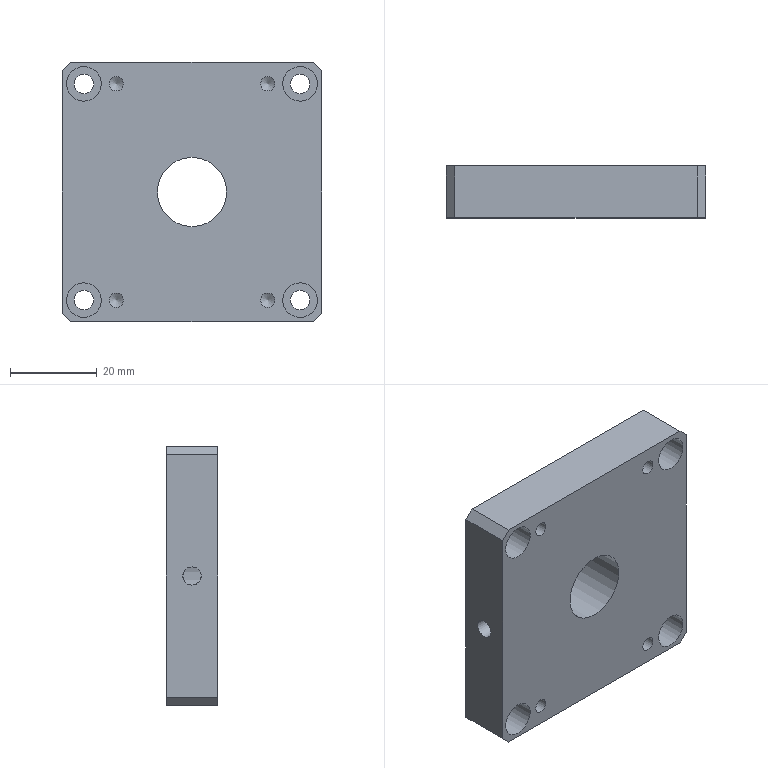CAM job | NX | 3+2 milling, drilling | part box 60 x 12 x 60 mm | stock box 60 x 12 x 60 mm
Tools:
number,name,description,diameter,corner_radius,flute_length,length,flutes
4,D4,平底铣刀-粗,4.0,0.0,25.0,75.0,2
9,D10,平底铣刀-粗,10.0,0.0,35.0,75.0,2
18,D1.5-J,平底铣刀-粗,1.5,0.0,50.0,75.0,2
11,D4-J,平底铣刀-精,4.0,0.0,50.0,75.0,2
10,D10-J,平底铣刀-精,10.0,0.0,35.0,75.0,2
2,D6倒角刀,倒角刀,6.0,0.0,3.0,25.0,2
21,M4X0.7,丝锥,3.3,0.0,35.0,50.0,2
1,C6定点钻,倒角刀,6.0,0.0,3.0,3.0,2
17,ZT1.8,钻头,1.6,0.0,35.0,50.0,2
13,ZT3.4,钻头,3.4,0.0,35.0,50.0,2
11,ZT4.5,钻头,4.5,0.0,35.0,50.0,2
Operations:
program,operation,operation_type,tool,method,geometry_group,spindle_rpm,surface_speed,feed_per_tooth,feed_cut,feed_plunge,cut_length_mm,path_length_mm,cut_time_min,machine_time_min
B,打点-深1_COPY,Operation,C6定点钻,NONE,W-B,3000.0,56.0,0.01,60.0,90.0,3.6,157.71,0.06,0.0754
B,盲锥孔-1-2,Operation,ZT1.8,NONE,W-B,2000.0,12.566,0.0075,30.0,90.0,13.202,176.913,0.4401,0.4564
B,底壁铣螺旋开粗-小_COPY,VolumeBased25DMillingOperation,D1.5-J,分层开粗-切深K-步距G,W-B,6000.0,28.274,0.0167,200.0,100.0,1219.408,1476.121,6.097,6.123
B,NG_钻倒角_2,Operation,D6倒角刀,METHOD,W-B,2000.0,0.0,0.025,100.0,0.0,22.2,303.67,0.222,0.2501
B,平面去毛刺6X45L_COPY_1,SurfaceContour,D6倒角刀,爬面_倒角-切深0-步距G,W-B,3500.0,65.972,0.1429,1000.0,100.0,345.537,759.417,0.3455,0.3869
B,NG_钻倒角_3,Operation,D6倒角刀,METHOD,W-B,4000.0,75.398,0.01,80.0,0.0,4.3,108.6,0.0537,0.0642
B,底壁铣螺旋精光-小_COPY,VolumeBased25DMillingOperation,D1.5-J,螺旋精光-切深K-步距G,W-B,6000.0,28.274,0.0167,200.0,100.0,164.905,421.703,0.8245,0.8502
A,打点-深0.8,Operation,C6定点钻,NONE,W-A,3000.0,56.0,0.01,60.0,90.0,16.2,311.433,0.27,0.2995
A,盲锥孔-M4螺纹底孔,Operation,ZT3.4,NONE,W-A,1500.0,16.022,0.0133,40.0,90.0,48.0,319.039,1.2,1.227
A,沉头孔-钻孔0段,Operation,ZT4.5,NONE,W-A,800.0,11.31,0.025,40.0,90.0,65.408,383.846,1.635,1.667
A,铣孔开粗D4_1,CylinderMilling,D4,NONE,W-A,4000.0,50.266,0.15,1200.0,100.0,1862.587,2438.587,1.552,1.61
A,铣孔精光D4_1,CylinderMilling,D4-J,精光步距切深关,W-A,4000.0,50.266,0.1,800.0,100.0,156.315,732.316,0.1954,0.253
A,铣孔开粗D8_1,CylinderMilling,D10,NONE,W-A,4000.0,125.664,0.15,1200.0,100.0,1232.674,1344.674,1.027,1.038
A,NG_钻倒角_1,Operation,D6倒角刀,METHOD,W-A,4000.0,75.398,0.01,80.0,0.0,20.8,270.947,0.26,0.285
A,铣倒角_1,PlanarMilling,D6倒角刀,NONE,W-A,4000.0,75.398,0.0625,500.0,100.0,135.871,677.194,0.2717,0.3259
A,平面去毛刺6X45L_COPY,SurfaceContour,D6倒角刀,爬面_倒角-切深0-步距G,W-A,3500.0,65.972,0.1429,1000.0,100.0,416.237,831.548,0.4162,0.4578
A,盲锥孔-攻牙M4,Operation,M4X0.7,METHOD,W-A,600.0,6.22,0.0006,0.7,90.0,36.4,295.839,52.0,52.026
A,底壁铣精光侧面-中_COPY,VolumeBased25DMillingOperation,D10-J,侧刃精光-切深K-步距G,W-A,3000.0,94.248,0.1333,800.0,100.0,60.723,102.806,0.0759,0.0801